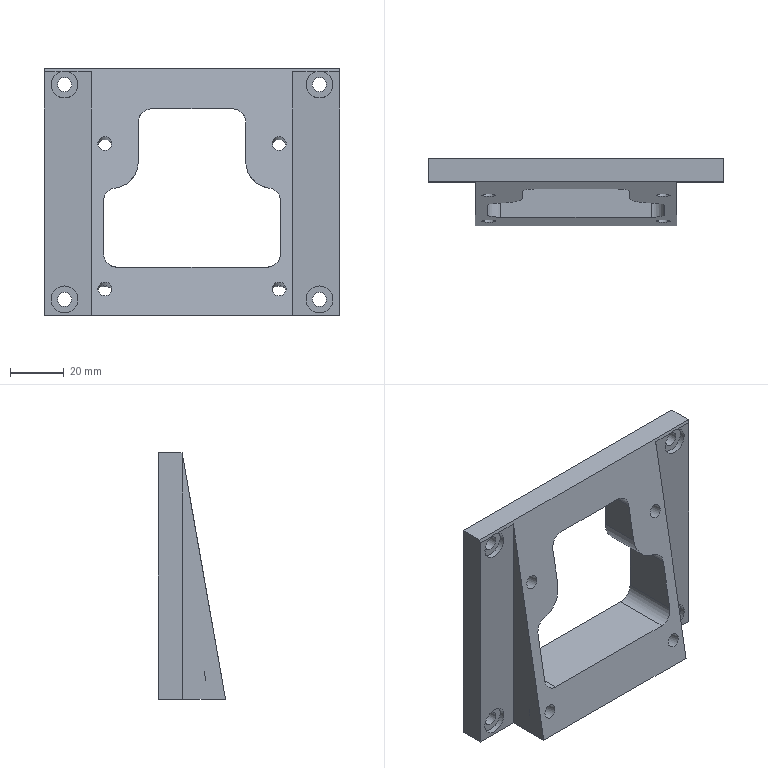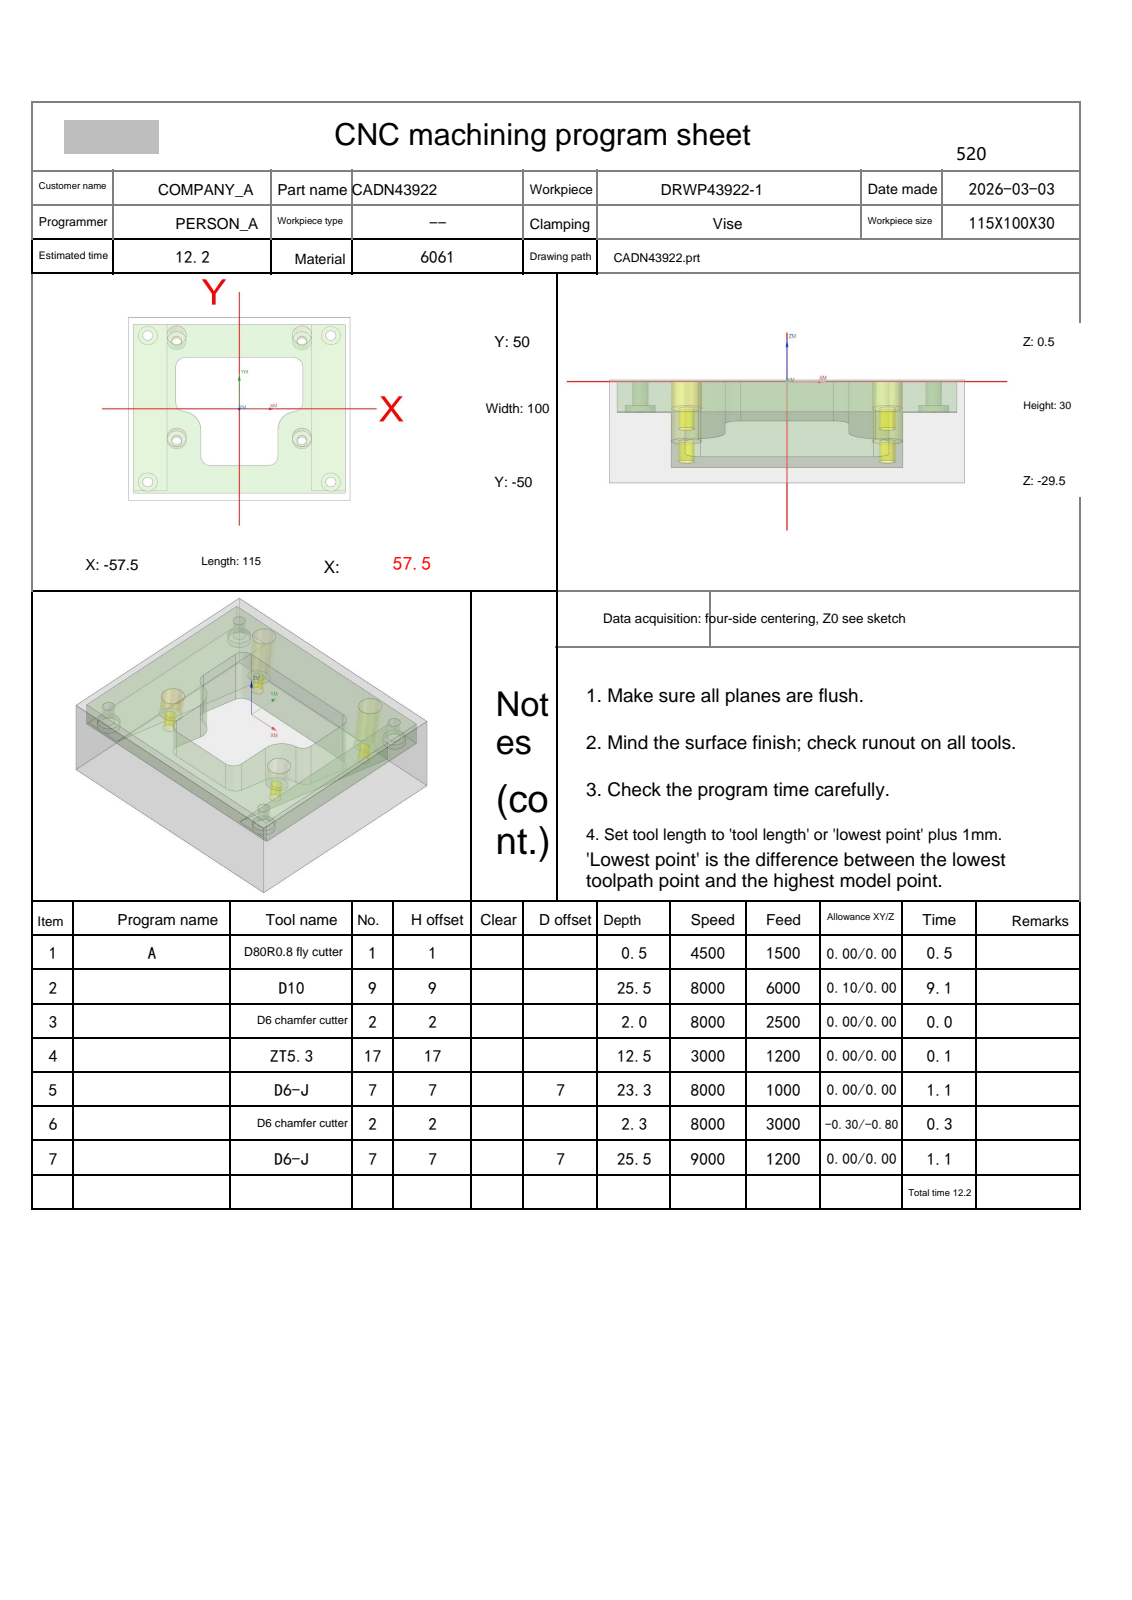NC program | NX | posted by the shop | part box 110 x 25 x 92 mm
Lines 1 to 35 of 4607:
%
O0001
(Machine time: 13.58 MIN)
(===Total Tool:5===)
(T1=D80R0.8 fly cutter D=80.  R=0.8  D-  H01 Z=0.    )
(T9=D10     D=10.  R=0.   D-  H09 Z=-25.  )
(T2=D6 chamfer cutter   D=6.   R=0.   D-  H02 Z=-1.8  )
(T17=ZT5.3  D=5.3  DR_a=118 D-  H17 Z=-12.  )
(T7=D6-J    D=6.   R=0.   D7  H07 Z=-25.  )
G80 G90 G17 G49 G40
G91 G28 Z0
M01
N1 T01 M06
(D80R0.8 fly cutter  D=80. R=0.8 H=01 ce=0.00 di=0.00)
G00 G90 G54 X100. Y-43. M03 S4500
G43 H01 Z50.
M08
Z2.
G01 Z0.0 F1500.
X95.
X-95.
Y0.0
X95.
Y43.
X-95.
X-100.
Z2.
G00 Z50.
G91 G28 Z0.0
M05
M09
G91 G28 Z0.0
M01